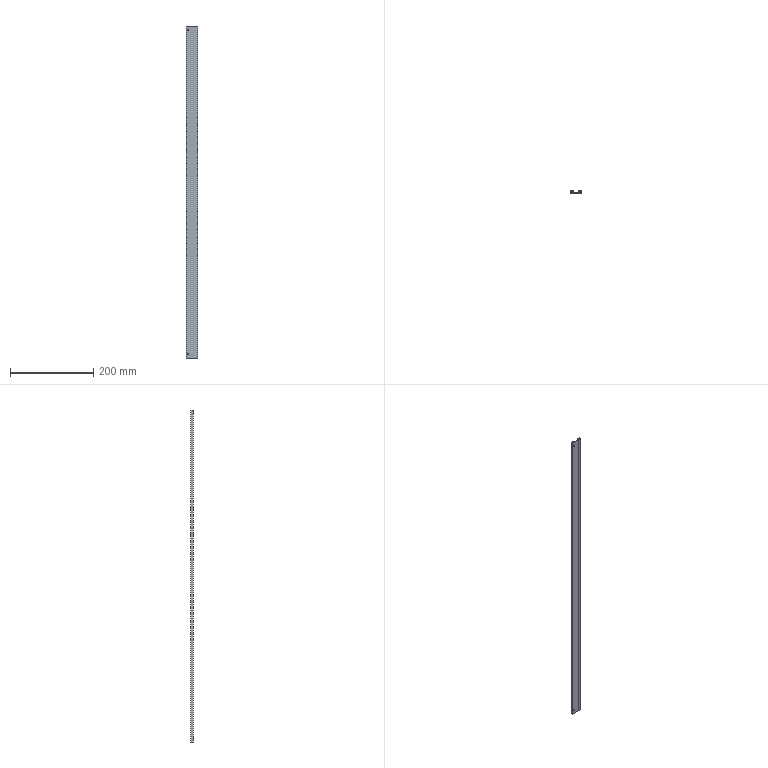Part | SolidWorks | features BossThin 1, ExtruThin 1, HoleWzd 1, MirrorSolid 1 | 1 solid | 30 faces | box 28 x 5 x 800 mm | volume 39502 mm3 | plane 26 | cylinder 4 | commonest cylinder face diameters 3.4 x4
STEP:
#1=CARTESIAN_POINT('',(-16.,0.,11.7));
#2=VERTEX_POINT('',#1);
#3=CARTESIAN_POINT('',(-16.,0.,8.3));
#4=VERTEX_POINT('',#3);
#5=CARTESIAN_POINT('',(-16.,0.,10.));
#6=DIRECTION('',(0.,-1.,0.));
#7=DIRECTION('',(0.,0.,-1.));
#8=AXIS2_PLACEMENT_3D('',#5,#6,#7);
#9=CIRCLE('',#8,1.7);
#10=EDGE_CURVE('',#2,#4,#9,.T.);
#11=ORIENTED_EDGE('',*,*,#10,.T.);
#12=CARTESIAN_POINT('',(-16.,1.,8.3));
#13=VERTEX_POINT('',#12);
#14=CARTESIAN_POINT('',(-16.,1.,8.3));
#15=DIRECTION('',(0.,1.,0.));
#16=VECTOR('',#15,1000.);
#17=LINE('',#14,#16);
#18=EDGE_CURVE('',#4,#13,#17,.T.);
#19=ORIENTED_EDGE('',*,*,#18,.T.);
#20=CARTESIAN_POINT('',(-16.,1.,11.7));
#21=VERTEX_POINT('',#20);
#22=CARTESIAN_POINT('',(-16.,1.,10.));
#23=DIRECTION('',(0.,1.,0.));
#24=DIRECTION('',(0.,0.,1.));
#25=AXIS2_PLACEMENT_3D('',#22,#23,#24);
#26=CIRCLE('',#25,1.7);
#27=EDGE_CURVE('',#13,#21,#26,.T.);
#28=ORIENTED_EDGE('',*,*,#27,.T.);
#29=CARTESIAN_POINT('',(-16.,1.,11.7));
#30=DIRECTION('',(0.,1.,0.));
#31=VECTOR('',#30,1000.);
#32=LINE('',#29,#31);
#33=EDGE_CURVE('',#2,#21,#32,.T.);
#34=ORIENTED_EDGE('',*,*,#33,.F.);
#35=EDGE_LOOP('',(#11,#19,#28,#34));
#36=FACE_OUTER_BOUND('',#35,.T.);
#37=CARTESIAN_POINT('',(-16.,1.,10.));
#38=DIRECTION('',(0.,1.,0.));
#39=DIRECTION('',(0.,0.,1.));
#40=AXIS2_PLACEMENT_3D('',#37,#38,#39);
#41=CYLINDRICAL_SURFACE('',#40,1.7);
#42=ADVANCED_FACE('',(#36),#41,.F.);
#43=CARTESIAN_POINT('',(-16.,0.,791.7));
#44=VERTEX_POINT('',#43);
#45=CARTESIAN_POINT('',(-16.,0.,788.3));
#46=VERTEX_POINT('',#45);
#47=CARTESIAN_POINT('',(-16.,0.,790.));
#48=DIRECTION('',(0.,-1.,0.));
#49=DIRECTION('',(0.,0.,-1.));
#50=AXIS2_PLACEMENT_3D('',#47,#48,#49);
#51=CIRCLE('',#50,1.7);
#52=EDGE_CURVE('',#44,#46,#51,.T.);
#53=ORIENTED_EDGE('',*,*,#52,.T.);
#54=CARTESIAN_POINT('',(-16.,1.,788.3));
#55=VERTEX_POINT('',#54);
#56=CARTESIAN_POINT('',(-16.,1.,788.3));
#57=DIRECTION('',(0.,1.,0.));
#58=VECTOR('',#57,1000.);
#59=LINE('',#56,#58);
#60=EDGE_CURVE('',#46,#55,#59,.T.);
#61=ORIENTED_EDGE('',*,*,#60,.T.);
#62=CARTESIAN_POINT('',(-16.,1.,791.7));
#63=VERTEX_POINT('',#62);
#64=CARTESIAN_POINT('',(-16.,1.,790.));
#65=DIRECTION('',(0.,1.,0.));
#66=DIRECTION('',(0.,0.,1.));
#67=AXIS2_PLACEMENT_3D('',#64,#65,#66);
#68=CIRCLE('',#67,1.7);
#69=EDGE_CURVE('',#55,#63,#68,.T.);
#70=ORIENTED_EDGE('',*,*,#69,.T.);
#71=CARTESIAN_POINT('',(-16.,1.,791.7));
#72=DIRECTION('',(0.,1.,0.));
#73=VECTOR('',#72,1000.);
#74=LINE('',#71,#73);
#75=EDGE_CURVE('',#44,#63,#74,.T.);
#76=ORIENTED_EDGE('',*,*,#75,.F.);
#77=EDGE_LOOP('',(#53,#61,#70,#76));
#78=FACE_OUTER_BOUND('',#77,.T.);
#79=CARTESIAN_POINT('',(-16.,1.,790.));
#80=DIRECTION('',(0.,1.,0.));
#81=DIRECTION('',(0.,0.,1.));
#82=AXIS2_PLACEMENT_3D('',#79,#80,#81);
#83=CYLINDRICAL_SURFACE('',#82,1.7);
#84=ADVANCED_FACE('',(#78),#83,.F.);
#85=CARTESIAN_POINT('',(0.,1.,0.));
#86=VERTEX_POINT('',#85);
#87=CARTESIAN_POINT('',(0.,5.,0.));
#88=VERTEX_POINT('',#87);
#89=CARTESIAN_POINT('',(0.,0.,0.));
#90=DIRECTION('',(0.,1.,0.));
#91=VECTOR('',#90,1000.);
#92=LINE('',#89,#91);
#93=EDGE_CURVE('',#86,#88,#92,.T.);
#94=ORIENTED_EDGE('',*,*,#93,.F.);
#95=CARTESIAN_POINT('',(0.,1.,800.));
#96=VERTEX_POINT('',#95);
#97=CARTESIAN_POINT('',(0.,1.,-6.083));
#98=DIRECTION('',(0.,0.,1.));
#99=VECTOR('',#98,1000.);
#100=LINE('',#97,#99);
#101=EDGE_CURVE('',#86,#96,#100,.T.);
#102=ORIENTED_EDGE('',*,*,#101,.T.);
#103=CARTESIAN_POINT('',(0.,5.,800.));
#104=VERTEX_POINT('',#103);
#105=CARTESIAN_POINT('',(0.,0.,800.));
#106=DIRECTION('',(0.,1.,0.));
#107=VECTOR('',#106,1000.);
#108=LINE('',#105,#107);
#109=EDGE_CURVE('',#96,#104,#108,.T.);
#110=ORIENTED_EDGE('',*,*,#109,.T.);
#111=CARTESIAN_POINT('',(0.,5.,800.));
#112=DIRECTION('',(0.,0.,-1.));
#113=VECTOR('',#112,1000.);
#114=LINE('',#111,#113);
#115=EDGE_CURVE('',#104,#88,#114,.T.);
#116=ORIENTED_EDGE('',*,*,#115,.T.);
#117=EDGE_LOOP('',(#94,#102,#110,#116));
#118=FACE_OUTER_BOUND('',#117,.T.);
#119=CARTESIAN_POINT('',(0.,0.,800.));
#120=DIRECTION('',(-1.,0.,0.));
#121=DIRECTION('',(0.,0.,1.));
#122=AXIS2_PLACEMENT_3D('',#119,#120,#121);
#123=PLANE('',#122);
#124=ADVANCED_FACE('',(#118),#123,.T.);
#125=CARTESIAN_POINT('',(1.,4.,0.));
#126=VERTEX_POINT('',#125);
#127=CARTESIAN_POINT('',(2.35,4.,0.));
#128=VERTEX_POINT('',#127);
#129=CARTESIAN_POINT('',(0.,4.,0.));
#130=DIRECTION('',(1.,0.,0.));
#131=VECTOR('',#130,1000.);
#132=LINE('',#129,#131);
#133=EDGE_CURVE('',#126,#128,#132,.T.);
#134=ORIENTED_EDGE('',*,*,#133,.T.);
#135=CARTESIAN_POINT('',(2.35,4.,800.));
#136=VERTEX_POINT('',#135);
#137=CARTESIAN_POINT('',(2.35,4.,800.));
#138=DIRECTION('',(0.,0.,-1.));
#139=VECTOR('',#138,1000.);
#140=LINE('',#137,#139);
#141=EDGE_CURVE('',#136,#128,#140,.T.);
#142=ORIENTED_EDGE('',*,*,#141,.F.);
#143=CARTESIAN_POINT('',(1.,4.,800.));
#144=VERTEX_POINT('',#143);
#145=CARTESIAN_POINT('',(0.,4.,800.));
#146=DIRECTION('',(1.,0.,0.));
#147=VECTOR('',#146,1000.);
#148=LINE('',#145,#147);
#149=EDGE_CURVE('',#144,#136,#148,.T.);
#150=ORIENTED_EDGE('',*,*,#149,.F.);
#151=CARTESIAN_POINT('',(1.,4.,800.));
#152=DIRECTION('',(0.,0.,-1.));
#153=VECTOR('',#152,1000.);
#154=LINE('',#151,#153);
#155=EDGE_CURVE('',#144,#126,#154,.T.);
#156=ORIENTED_EDGE('',*,*,#155,.T.);
#157=EDGE_LOOP('',(#134,#142,#150,#156));
#158=FACE_OUTER_BOUND('',#157,.T.);
#159=CARTESIAN_POINT('',(0.,4.,800.));
#160=DIRECTION('',(0.,1.,0.));
#161=DIRECTION('',(-1.,0.,0.));
#162=AXIS2_PLACEMENT_3D('',#159,#160,#161);
#163=PLANE('',#162);
#164=ADVANCED_FACE('',(#158),#163,.F.);
#165=CARTESIAN_POINT('',(2.35,5.,0.));
#166=VERTEX_POINT('',#165);
#167=CARTESIAN_POINT('',(2.35,5.,0.));
#168=DIRECTION('',(0.,-1.,0.));
#169=VECTOR('',#168,1000.);
#170=LINE('',#167,#169);
#171=EDGE_CURVE('',#166,#128,#170,.T.);
#172=ORIENTED_EDGE('',*,*,#171,.F.);
#173=CARTESIAN_POINT('',(2.35,5.,800.));
#174=VERTEX_POINT('',#173);
#175=CARTESIAN_POINT('',(2.35,5.,800.));
#176=DIRECTION('',(0.,0.,-1.));
#177=VECTOR('',#176,1000.);
#178=LINE('',#175,#177);
#179=EDGE_CURVE('',#174,#166,#178,.T.);
#180=ORIENTED_EDGE('',*,*,#179,.F.);
#181=CARTESIAN_POINT('',(2.35,5.,800.));
#182=DIRECTION('',(0.,-1.,0.));
#183=VECTOR('',#182,1000.);
#184=LINE('',#181,#183);
#185=EDGE_CURVE('',#174,#136,#184,.T.);
#186=ORIENTED_EDGE('',*,*,#185,.T.);
#187=ORIENTED_EDGE('',*,*,#141,.T.);
#188=EDGE_LOOP('',(#172,#180,#186,#187));
#189=FACE_OUTER_BOUND('',#188,.T.);
#190=CARTESIAN_POINT('',(2.35,5.,800.));
#191=DIRECTION('',(1.,0.,0.));
#192=DIRECTION('',(0.,1.,0.));
#193=AXIS2_PLACEMENT_3D('',#190,#191,#192);
#194=PLANE('',#193);
#195=ADVANCED_FACE('',(#189),#194,.T.);
#196=CARTESIAN_POINT('',(0.,5.,0.));
#197=DIRECTION('',(1.,0.,0.));
#198=VECTOR('',#197,1000.);
#199=LINE('',#196,#198);
#200=EDGE_CURVE('',#88,#166,#199,.T.);
#201=ORIENTED_EDGE('',*,*,#200,.F.);
#202=ORIENTED_EDGE('',*,*,#115,.F.);
#203=CARTESIAN_POINT('',(0.,5.,800.));
#204=DIRECTION('',(1.,0.,0.));
#205=VECTOR('',#204,1000.);
#206=LINE('',#203,#205);
#207=EDGE_CURVE('',#104,#174,#206,.T.);
#208=ORIENTED_EDGE('',*,*,#207,.T.);
#209=ORIENTED_EDGE('',*,*,#179,.T.);
#210=EDGE_LOOP('',(#201,#202,#208,#209));
#211=FACE_OUTER_BOUND('',#210,.T.);
#212=CARTESIAN_POINT('',(0.,5.,800.));
#213=DIRECTION('',(0.,1.,0.));
#214=DIRECTION('',(-1.,0.,0.));
#215=AXIS2_PLACEMENT_3D('',#212,#213,#214);
#216=PLANE('',#215);
#217=ADVANCED_FACE('',(#211),#216,.T.);
#218=ORIENTED_EDGE('',*,*,#10,.F.);
#219=CARTESIAN_POINT('',(-16.,0.,10.));
#220=DIRECTION('',(0.,-1.,0.));
#221=DIRECTION('',(0.,0.,-1.));
#222=AXIS2_PLACEMENT_3D('',#219,#220,#221);
#223=CIRCLE('',#222,1.7);
#224=EDGE_CURVE('',#4,#2,#223,.T.);
#225=ORIENTED_EDGE('',*,*,#224,.F.);
#226=EDGE_LOOP('',(#218,#225));
#227=FACE_BOUND('',#226,.T.);
#228=ORIENTED_EDGE('',*,*,#52,.F.);
#229=CARTESIAN_POINT('',(-16.,0.,790.));
#230=DIRECTION('',(0.,-1.,0.));
#231=DIRECTION('',(0.,0.,-1.));
#232=AXIS2_PLACEMENT_3D('',#229,#230,#231);
#233=CIRCLE('',#232,1.7);
#234=EDGE_CURVE('',#46,#44,#233,.T.);
#235=ORIENTED_EDGE('',*,*,#234,.F.);
#236=EDGE_LOOP('',(#228,#235));
#237=FACE_BOUND('',#236,.T.);
#238=CARTESIAN_POINT('',(8.,0.,0.));
#239=VERTEX_POINT('',#238);
#240=CARTESIAN_POINT('',(-20.,0.,0.));
#241=VERTEX_POINT('',#240);
#242=CARTESIAN_POINT('',(0.,0.,0.));
#243=DIRECTION('',(-1.,0.,0.));
#244=VECTOR('',#243,1000.);
#245=LINE('',#242,#244);
#246=EDGE_CURVE('',#239,#241,#245,.T.);
#247=ORIENTED_EDGE('',*,*,#246,.F.);
#248=CARTESIAN_POINT('',(8.,0.,800.));
#249=VERTEX_POINT('',#248);
#250=CARTESIAN_POINT('',(8.,0.,800.));
#251=DIRECTION('',(0.,0.,-1.));
#252=VECTOR('',#251,1000.);
#253=LINE('',#250,#252);
#254=EDGE_CURVE('',#249,#239,#253,.T.);
#255=ORIENTED_EDGE('',*,*,#254,.F.);
#256=CARTESIAN_POINT('',(-20.,0.,800.));
#257=VERTEX_POINT('',#256);
#258=CARTESIAN_POINT('',(0.,0.,800.));
#259=DIRECTION('',(-1.,0.,0.));
#260=VECTOR('',#259,1000.);
#261=LINE('',#258,#260);
#262=EDGE_CURVE('',#249,#257,#261,.T.);
#263=ORIENTED_EDGE('',*,*,#262,.T.);
#264=CARTESIAN_POINT('',(-20.,0.,800.));
#265=DIRECTION('',(0.,0.,-1.));
#266=VECTOR('',#265,1000.);
#267=LINE('',#264,#266);
#268=EDGE_CURVE('',#257,#241,#267,.T.);
#269=ORIENTED_EDGE('',*,*,#268,.T.);
#270=EDGE_LOOP('',(#247,#255,#263,#269));
#271=FACE_OUTER_BOUND('',#270,.T.);
#272=CARTESIAN_POINT('',(0.,0.,800.));
#273=DIRECTION('',(0.,-1.,0.));
#274=DIRECTION('',(0.,0.,-1.));
#275=AXIS2_PLACEMENT_3D('',#272,#273,#274);
#276=PLANE('',#275);
#277=ADVANCED_FACE('',(#227,#237,#271),#276,.T.);
#278=CARTESIAN_POINT('',(8.,5.,0.));
#279=VERTEX_POINT('',#278);
#280=CARTESIAN_POINT('',(8.,0.,0.));
#281=DIRECTION('',(0.,-1.,0.));
#282=VECTOR('',#281,1000.);
#283=LINE('',#280,#282);
#284=EDGE_CURVE('',#279,#239,#283,.T.);
#285=ORIENTED_EDGE('',*,*,#284,.F.);
#286=CARTESIAN_POINT('',(8.,5.,800.));
#287=VERTEX_POINT('',#286);
#288=CARTESIAN_POINT('',(8.,5.,800.));
#289=DIRECTION('',(0.,0.,-1.));
#290=VECTOR('',#289,1000.);
#291=LINE('',#288,#290);
#292=EDGE_CURVE('',#287,#279,#291,.T.);
#293=ORIENTED_EDGE('',*,*,#292,.F.);
#294=CARTESIAN_POINT('',(8.,0.,800.));
#295=DIRECTION('',(0.,-1.,0.));
#296=VECTOR('',#295,1000.);
#297=LINE('',#294,#296);
#298=EDGE_CURVE('',#287,#249,#297,.T.);
#299=ORIENTED_EDGE('',*,*,#298,.T.);
#300=ORIENTED_EDGE('',*,*,#254,.T.);
#301=EDGE_LOOP('',(#285,#293,#299,#300));
#302=FACE_OUTER_BOUND('',#301,.T.);
#303=CARTESIAN_POINT('',(8.,0.,800.));
#304=DIRECTION('',(1.,0.,0.));
#305=DIRECTION('',(0.,0.,-1.));
#306=AXIS2_PLACEMENT_3D('',#303,#304,#305);
#307=PLANE('',#306);
#308=ADVANCED_FACE('',(#302),#307,.T.);
#309=CARTESIAN_POINT('',(5.65,5.,0.));
#310=VERTEX_POINT('',#309);
#311=CARTESIAN_POINT('',(8.,5.,0.));
#312=DIRECTION('',(1.,0.,0.));
#313=VECTOR('',#312,1000.);
#314=LINE('',#311,#313);
#315=EDGE_CURVE('',#310,#279,#314,.T.);
#316=ORIENTED_EDGE('',*,*,#315,.F.);
#317=CARTESIAN_POINT('',(5.65,5.,800.));
#318=VERTEX_POINT('',#317);
#319=CARTESIAN_POINT('',(5.65,5.,800.));
#320=DIRECTION('',(0.,0.,-1.));
#321=VECTOR('',#320,1000.);
#322=LINE('',#319,#321);
#323=EDGE_CURVE('',#318,#310,#322,.T.);
#324=ORIENTED_EDGE('',*,*,#323,.F.);
#325=CARTESIAN_POINT('',(8.,5.,800.));
#326=DIRECTION('',(1.,0.,0.));
#327=VECTOR('',#326,1000.);
#328=LINE('',#325,#327);
#329=EDGE_CURVE('',#318,#287,#328,.T.);
#330=ORIENTED_EDGE('',*,*,#329,.T.);
#331=ORIENTED_EDGE('',*,*,#292,.T.);
#332=EDGE_LOOP('',(#316,#324,#330,#331));
#333=FACE_OUTER_BOUND('',#332,.T.);
#334=CARTESIAN_POINT('',(8.,5.,800.));
#335=DIRECTION('',(0.,1.,0.));
#336=DIRECTION('',(-1.,0.,0.));
#337=AXIS2_PLACEMENT_3D('',#334,#335,#336);
#338=PLANE('',#337);
#339=ADVANCED_FACE('',(#333),#338,.T.);
#340=CARTESIAN_POINT('',(5.65,4.,0.));
#341=VERTEX_POINT('',#340);
#342=CARTESIAN_POINT('',(5.65,4.,0.));
#343=DIRECTION('',(0.,1.,0.));
#344=VECTOR('',#343,1000.);
#345=LINE('',#342,#344);
#346=EDGE_CURVE('',#341,#310,#345,.T.);
#347=ORIENTED_EDGE('',*,*,#346,.F.);
#348=CARTESIAN_POINT('',(5.65,4.,800.));
#349=VERTEX_POINT('',#348);
#350=CARTESIAN_POINT('',(5.65,4.,800.));
#351=DIRECTION('',(0.,0.,-1.));
#352=VECTOR('',#351,1000.);
#353=LINE('',#350,#352);
#354=EDGE_CURVE('',#349,#341,#353,.T.);
#355=ORIENTED_EDGE('',*,*,#354,.F.);
#356=CARTESIAN_POINT('',(5.65,4.,800.));
#357=DIRECTION('',(0.,1.,0.));
#358=VECTOR('',#357,1000.);
#359=LINE('',#356,#358);
#360=EDGE_CURVE('',#349,#318,#359,.T.);
#361=ORIENTED_EDGE('',*,*,#360,.T.);
#362=ORIENTED_EDGE('',*,*,#323,.T.);
#363=EDGE_LOOP('',(#347,#355,#361,#362));
#364=FACE_OUTER_BOUND('',#363,.T.);
#365=CARTESIAN_POINT('',(5.65,4.,800.));
#366=DIRECTION('',(-1.,0.,0.));
#367=DIRECTION('',(0.,0.,1.));
#368=AXIS2_PLACEMENT_3D('',#365,#366,#367);
#369=PLANE('',#368);
#370=ADVANCED_FACE('',(#364),#369,.T.);
#371=CARTESIAN_POINT('',(7.,4.,0.));
#372=VERTEX_POINT('',#371);
#373=CARTESIAN_POINT('',(8.,4.,0.));
#374=DIRECTION('',(1.,0.,0.));
#375=VECTOR('',#374,1000.);
#376=LINE('',#373,#375);
#377=EDGE_CURVE('',#341,#372,#376,.T.);
#378=ORIENTED_EDGE('',*,*,#377,.T.);
#379=CARTESIAN_POINT('',(7.,4.,800.));
#380=VERTEX_POINT('',#379);
#381=CARTESIAN_POINT('',(7.,4.,800.));
#382=DIRECTION('',(0.,0.,-1.));
#383=VECTOR('',#382,1000.);
#384=LINE('',#381,#383);
#385=EDGE_CURVE('',#380,#372,#384,.T.);
#386=ORIENTED_EDGE('',*,*,#385,.F.);
#387=CARTESIAN_POINT('',(8.,4.,800.));
#388=DIRECTION('',(1.,0.,0.));
#389=VECTOR('',#388,1000.);
#390=LINE('',#387,#389);
#391=EDGE_CURVE('',#349,#380,#390,.T.);
#392=ORIENTED_EDGE('',*,*,#391,.F.);
#393=ORIENTED_EDGE('',*,*,#354,.T.);
#394=EDGE_LOOP('',(#378,#386,#392,#393));
#395=FACE_OUTER_BOUND('',#394,.T.);
#396=CARTESIAN_POINT('',(8.,4.,800.));
#397=DIRECTION('',(0.,1.,0.));
#398=DIRECTION('',(-1.,0.,0.));
#399=AXIS2_PLACEMENT_3D('',#396,#397,#398);
#400=PLANE('',#399);
#401=ADVANCED_FACE('',(#395),#400,.F.);
#402=CARTESIAN_POINT('',(7.,1.,0.));
#403=VERTEX_POINT('',#402);
#404=CARTESIAN_POINT('',(7.,0.,0.));
#405=DIRECTION('',(0.,-1.,0.));
#406=VECTOR('',#405,1000.);
#407=LINE('',#404,#406);
#408=EDGE_CURVE('',#372,#403,#407,.T.);
#409=ORIENTED_EDGE('',*,*,#408,.T.);
#410=CARTESIAN_POINT('',(7.,1.,800.));
#411=VERTEX_POINT('',#410);
#412=CARTESIAN_POINT('',(7.,1.,800.));
#413=DIRECTION('',(0.,0.,-1.));
#414=VECTOR('',#413,1000.);
#415=LINE('',#412,#414);
#416=EDGE_CURVE('',#411,#403,#415,.T.);
#417=ORIENTED_EDGE('',*,*,#416,.F.);
#418=CARTESIAN_POINT('',(7.,0.,800.));
#419=DIRECTION('',(0.,-1.,0.));
#420=VECTOR('',#419,1000.);
#421=LINE('',#418,#420);
#422=EDGE_CURVE('',#380,#411,#421,.T.);
#423=ORIENTED_EDGE('',*,*,#422,.F.);
#424=ORIENTED_EDGE('',*,*,#385,.T.);
#425=EDGE_LOOP('',(#409,#417,#423,#424));
#426=FACE_OUTER_BOUND('',#425,.T.);
#427=CARTESIAN_POINT('',(7.,0.,800.));
#428=DIRECTION('',(1.,0.,0.));
#429=DIRECTION('',(0.,0.,-1.));
#430=AXIS2_PLACEMENT_3D('',#427,#428,#429);
#431=PLANE('',#430);
#432=ADVANCED_FACE('',(#426),#431,.F.);
#433=CARTESIAN_POINT('',(1.,1.,0.));
#434=VERTEX_POINT('',#433);
#435=CARTESIAN_POINT('',(0.,1.,0.));
#436=DIRECTION('',(-1.,0.,0.));
#437=VECTOR('',#436,1000.);
#438=LINE('',#435,#437);
#439=EDGE_CURVE('',#403,#434,#438,.T.);
#440=ORIENTED_EDGE('',*,*,#439,.T.);
#441=CARTESIAN_POINT('',(1.,1.,800.));
#442=VERTEX_POINT('',#441);
#443=CARTESIAN_POINT('',(1.,1.,800.));
#444=DIRECTION('',(0.,0.,-1.));
#445=VECTOR('',#444,1000.);
#446=LINE('',#443,#445);
#447=EDGE_CURVE('',#442,#434,#446,.T.);
#448=ORIENTED_EDGE('',*,*,#447,.F.);
#449=CARTESIAN_POINT('',(0.,1.,800.));
#450=DIRECTION('',(-1.,0.,0.));
#451=VECTOR('',#450,1000.);
#452=LINE('',#449,#451);
#453=EDGE_CURVE('',#411,#442,#452,.T.);
#454=ORIENTED_EDGE('',*,*,#453,.F.);
#455=ORIENTED_EDGE('',*,*,#416,.T.);
#456=EDGE_LOOP('',(#440,#448,#454,#455));
#457=FACE_OUTER_BOUND('',#456,.T.);
#458=CARTESIAN_POINT('',(0.,1.,800.));
#459=DIRECTION('',(0.,-1.,0.));
#460=DIRECTION('',(0.,0.,-1.));
#461=AXIS2_PLACEMENT_3D('',#458,#459,#460);
#462=PLANE('',#461);
#463=ADVANCED_FACE('',(#457),#462,.F.);
#464=CARTESIAN_POINT('',(1.,0.,0.));
#465=DIRECTION('',(0.,1.,0.));
#466=VECTOR('',#465,1000.);
#467=LINE('',#464,#466);
#468=EDGE_CURVE('',#434,#126,#467,.T.);
#469=ORIENTED_EDGE('',*,*,#468,.T.);
#470=ORIENTED_EDGE('',*,*,#155,.F.);
#471=CARTESIAN_POINT('',(1.,0.,800.));
#472=DIRECTION('',(0.,1.,0.));
#473=VECTOR('',#472,1000.);
#474=LINE('',#471,#473);
#475=EDGE_CURVE('',#442,#144,#474,.T.);
#476=ORIENTED_EDGE('',*,*,#475,.F.);
#477=ORIENTED_EDGE('',*,*,#447,.T.);
#478=EDGE_LOOP('',(#469,#470,#476,#477));
#479=FACE_OUTER_BOUND('',#478,.T.);
#480=CARTESIAN_POINT('',(1.,0.,800.));
#481=DIRECTION('',(-1.,0.,0.));
#482=DIRECTION('',(0.,0.,1.));
#483=AXIS2_PLACEMENT_3D('',#480,#481,#482);
#484=PLANE('',#483);
#485=ADVANCED_FACE('',(#479),#484,.F.);
#486=ORIENTED_EDGE('',*,*,#149,.T.);
#487=ORIENTED_EDGE('',*,*,#185,.F.);
#488=ORIENTED_EDGE('',*,*,#207,.F.);
#489=ORIENTED_EDGE('',*,*,#109,.F.);
#490=CARTESIAN_POINT('',(-12.,1.,800.));
#491=VERTEX_POINT('',#490);
#492=CARTESIAN_POINT('',(0.,1.,800.));
#493=DIRECTION('',(-1.,0.,0.));
#494=VECTOR('',#493,1000.);
#495=LINE('',#492,#494);
#496=EDGE_CURVE('',#96,#491,#495,.T.);
#497=ORIENTED_EDGE('',*,*,#496,.T.);
#498=CARTESIAN_POINT('',(-12.,5.,800.));
#499=VERTEX_POINT('',#498);
#500=CARTESIAN_POINT('',(-12.,0.,800.));
#501=DIRECTION('',(0.,1.,0.));
#502=VECTOR('',#501,1000.);
#503=LINE('',#500,#502);
#504=EDGE_CURVE('',#491,#499,#503,.T.);
#505=ORIENTED_EDGE('',*,*,#504,.T.);
#506=CARTESIAN_POINT('',(-14.35,5.,800.));
#507=VERTEX_POINT('',#506);
#508=CARTESIAN_POINT('',(-12.,5.,800.));
#509=DIRECTION('',(-1.,0.,0.));
#510=VECTOR('',#509,1000.);
#511=LINE('',#508,#510);
#512=EDGE_CURVE('',#499,#507,#511,.T.);
#513=ORIENTED_EDGE('',*,*,#512,.T.);
#514=CARTESIAN_POINT('',(-14.35,4.,800.));
#515=VERTEX_POINT('',#514);
#516=CARTESIAN_POINT('',(-14.35,5.,800.));
#517=DIRECTION('',(0.,-1.,0.));
#518=VECTOR('',#517,1000.);
#519=LINE('',#516,#518);
#520=EDGE_CURVE('',#507,#515,#519,.T.);
#521=ORIENTED_EDGE('',*,*,#520,.T.);
#522=CARTESIAN_POINT('',(-13.,4.,800.));
#523=VERTEX_POINT('',#522);
#524=CARTESIAN_POINT('',(-12.,4.,800.));
#525=DIRECTION('',(-1.,0.,0.));
#526=VECTOR('',#525,1000.);
#527=LINE('',#524,#526);
#528=EDGE_CURVE('',#523,#515,#527,.T.);
#529=ORIENTED_EDGE('',*,*,#528,.F.);
#530=CARTESIAN_POINT('',(-13.,1.,800.));
#531=VERTEX_POINT('',#530);
#532=CARTESIAN_POINT('',(-13.,0.,800.));
#533=DIRECTION('',(0.,1.,0.));
#534=VECTOR('',#533,1000.);
#535=LINE('',#532,#534);
#536=EDGE_CURVE('',#531,#523,#535,.T.);
#537=ORIENTED_EDGE('',*,*,#536,.F.);
#538=CARTESIAN_POINT('',(-19.,1.,800.));
#539=VERTEX_POINT('',#538);
#540=CARTESIAN_POINT('',(-12.,1.,800.));
#541=DIRECTION('',(1.,0.,0.));
#542=VECTOR('',#541,1000.);
#543=LINE('',#540,#542);
#544=EDGE_CURVE('',#539,#531,#543,.T.);
#545=ORIENTED_EDGE('',*,*,#544,.F.);
#546=CARTESIAN_POINT('',(-19.,4.,800.));
#547=VERTEX_POINT('',#546);
#548=CARTESIAN_POINT('',(-19.,0.,800.));
#549=DIRECTION('',(0.,-1.,0.));
#550=VECTOR('',#549,1000.);
#551=LINE('',#548,#550);
#552=EDGE_CURVE('',#547,#539,#551,.T.);
#553=ORIENTED_EDGE('',*,*,#552,.F.);
#554=CARTESIAN_POINT('',(-17.65,4.,800.));
#555=VERTEX_POINT('',#554);
#556=CARTESIAN_POINT('',(-20.,4.,800.));
#557=DIRECTION('',(-1.,0.,0.));
#558=VECTOR('',#557,1000.);
#559=LINE('',#556,#558);
#560=EDGE_CURVE('',#555,#547,#559,.T.);
#561=ORIENTED_EDGE('',*,*,#560,.F.);
#562=CARTESIAN_POINT('',(-17.65,5.,800.));
#563=VERTEX_POINT('',#562);
#564=CARTESIAN_POINT('',(-17.65,4.,800.));
#565=DIRECTION('',(0.,1.,0.));
#566=VECTOR('',#565,1000.);
#567=LINE('',#564,#566);
#568=EDGE_CURVE('',#555,#563,#567,.T.);
#569=ORIENTED_EDGE('',*,*,#568,.T.);
#570=CARTESIAN_POINT('',(-20.,5.,800.));
#571=VERTEX_POINT('',#570);
#572=CARTESIAN_POINT('',(-20.,5.,800.));
#573=DIRECTION('',(-1.,0.,0.));
#574=VECTOR('',#573,1000.);
#575=LINE('',#572,#574);
#576=EDGE_CURVE('',#563,#571,#575,.T.);
#577=ORIENTED_EDGE('',*,*,#576,.T.);
#578=CARTESIAN_POINT('',(-20.,0.,800.));
#579=DIRECTION('',(0.,-1.,0.));
#580=VECTOR('',#579,1000.);
#581=LINE('',#578,#580);
#582=EDGE_CURVE('',#571,#257,#581,.T.);
#583=ORIENTED_EDGE('',*,*,#582,.T.);
#584=ORIENTED_EDGE('',*,*,#262,.F.);
#585=ORIENTED_EDGE('',*,*,#298,.F.);
#586=ORIENTED_EDGE('',*,*,#329,.F.);
#587=ORIENTED_EDGE('',*,*,#360,.F.);
#588=ORIENTED_EDGE('',*,*,#391,.T.);
#589=ORIENTED_EDGE('',*,*,#422,.T.);
#590=ORIENTED_EDGE('',*,*,#453,.T.);
#591=ORIENTED_EDGE('',*,*,#475,.T.);
#592=EDGE_LOOP('',(#486,#487,#488,#489,#497,#505,#513,#521,#529,#537,#545,#553,#561,#569,#577,#583,#584,#585,#586,#587,#588,#589,#590,#591));
#593=FACE_OUTER_BOUND('',#592,.T.);
#594=CARTESIAN_POINT('',(0.,0.,800.));
#595=DIRECTION('',(0.,0.,-1.));
#596=DIRECTION('',(-1.,0.,0.));
#597=AXIS2_PLACEMENT_3D('',#594,#595,#596);
#598=PLANE('',#597);
#599=ADVANCED_FACE('',(#593),#598,.F.);
#600=ORIENTED_EDGE('',*,*,#133,.F.);
#601=ORIENTED_EDGE('',*,*,#468,.F.);
#602=ORIENTED_EDGE('',*,*,#439,.F.);
#603=ORIENTED_EDGE('',*,*,#408,.F.);
#604=ORIENTED_EDGE('',*,*,#377,.F.);
#605=ORIENTED_EDGE('',*,*,#346,.T.);
#606=ORIENTED_EDGE('',*,*,#315,.T.);
#607=ORIENTED_EDGE('',*,*,#284,.T.);
#608=ORIENTED_EDGE('',*,*,#246,.T.);
#609=CARTESIAN_POINT('',(-20.,5.,0.));
#610=VERTEX_POINT('',#609);
#611=CARTESIAN_POINT('',(-20.,0.,0.));
#612=DIRECTION('',(0.,-1.,0.));
#613=VECTOR('',#612,1000.);
#614=LINE('',#611,#613);
#615=EDGE_CURVE('',#610,#241,#614,.T.);
#616=ORIENTED_EDGE('',*,*,#615,.F.);
#617=CARTESIAN_POINT('',(-17.65,5.,0.));
#618=VERTEX_POINT('',#617);
#619=CARTESIAN_POINT('',(-20.,5.,0.));
#620=DIRECTION('',(-1.,0.,0.));
#621=VECTOR('',#620,1000.);
#622=LINE('',#619,#621);
#623=EDGE_CURVE('',#618,#610,#622,.T.);
#624=ORIENTED_EDGE('',*,*,#623,.F.);
#625=CARTESIAN_POINT('',(-17.65,4.,0.));
#626=VERTEX_POINT('',#625);
#627=CARTESIAN_POINT('',(-17.65,4.,0.));
#628=DIRECTION('',(0.,1.,0.));
#629=VECTOR('',#628,1000.);
#630=LINE('',#627,#629);
#631=EDGE_CURVE('',#626,#618,#630,.T.);
#632=ORIENTED_EDGE('',*,*,#631,.F.);
#633=CARTESIAN_POINT('',(-19.,4.,0.));
#634=VERTEX_POINT('',#633);
#635=CARTESIAN_POINT('',(-20.,4.,0.));
#636=DIRECTION('',(-1.,0.,0.));
#637=VECTOR('',#636,1000.);
#638=LINE('',#635,#637);
#639=EDGE_CURVE('',#626,#634,#638,.T.);
#640=ORIENTED_EDGE('',*,*,#639,.T.);
#641=CARTESIAN_POINT('',(-19.,1.,0.));
#642=VERTEX_POINT('',#641);
#643=CARTESIAN_POINT('',(-19.,0.,0.));
#644=DIRECTION('',(0.,-1.,0.));
#645=VECTOR('',#644,1000.);
#646=LINE('',#643,#645);
#647=EDGE_CURVE('',#634,#642,#646,.T.);
#648=ORIENTED_EDGE('',*,*,#647,.T.);
#649=CARTESIAN_POINT('',(-13.,1.,0.));
#650=VERTEX_POINT('',#649);
#651=CARTESIAN_POINT('',(-12.,1.,0.));
#652=DIRECTION('',(1.,0.,0.));
#653=VECTOR('',#652,1000.);
#654=LINE('',#651,#653);
#655=EDGE_CURVE('',#642,#650,#654,.T.);
#656=ORIENTED_EDGE('',*,*,#655,.T.);
#657=CARTESIAN_POINT('',(-13.,4.,0.));
#658=VERTEX_POINT('',#657);
#659=CARTESIAN_POINT('',(-13.,0.,0.));
#660=DIRECTION('',(0.,1.,0.));
#661=VECTOR('',#660,1000.);
#662=LINE('',#659,#661);
#663=EDGE_CURVE('',#650,#658,#662,.T.);
#664=ORIENTED_EDGE('',*,*,#663,.T.);
#665=CARTESIAN_POINT('',(-14.35,4.,0.));
#666=VERTEX_POINT('',#665);
#667=CARTESIAN_POINT('',(-12.,4.,0.));
#668=DIRECTION('',(-1.,0.,0.));
#669=VECTOR('',#668,1000.);
#670=LINE('',#667,#669);
#671=EDGE_CURVE('',#658,#666,#670,.T.);
#672=ORIENTED_EDGE('',*,*,#671,.T.);
#673=CARTESIAN_POINT('',(-14.35,5.,0.));
#674=VERTEX_POINT('',#673);
#675=CARTESIAN_POINT('',(-14.35,5.,0.));
#676=DIRECTION('',(0.,-1.,0.));
#677=VECTOR('',#676,1000.);
#678=LINE('',#675,#677);
#679=EDGE_CURVE('',#674,#666,#678,.T.);
#680=ORIENTED_EDGE('',*,*,#679,.F.);
#681=CARTESIAN_POINT('',(-12.,5.,0.));
#682=VERTEX_POINT('',#681);
#683=CARTESIAN_POINT('',(-12.,5.,0.));
#684=DIRECTION('',(-1.,0.,0.));
#685=VECTOR('',#684,1000.);
#686=LINE('',#683,#685);
#687=EDGE_CURVE('',#682,#674,#686,.T.);
#688=ORIENTED_EDGE('',*,*,#687,.F.);
#689=CARTESIAN_POINT('',(-12.,1.,0.));
#690=VERTEX_POINT('',#689);
#691=CARTESIAN_POINT('',(-12.,0.,0.));
#692=DIRECTION('',(0.,1.,0.));
#693=VECTOR('',#692,1000.);
#694=LINE('',#691,#693);
#695=EDGE_CURVE('',#690,#682,#694,.T.);
#696=ORIENTED_EDGE('',*,*,#695,.F.);
#697=CARTESIAN_POINT('',(0.,1.,0.));
#698=DIRECTION('',(-1.,0.,0.));
#699=VECTOR('',#698,1000.);
#700=LINE('',#697,#699);
#701=EDGE_CURVE('',#86,#690,#700,.T.);
#702=ORIENTED_EDGE('',*,*,#701,.F.);
#703=ORIENTED_EDGE('',*,*,#93,.T.);
#704=ORIENTED_EDGE('',*,*,#200,.T.);
#705=ORIENTED_EDGE('',*,*,#171,.T.);
#706=EDGE_LOOP('',(#600,#601,#602,#603,#604,#605,#606,#607,#608,#616,#624,#632,#640,#648,#656,#664,#672,#680,#688,#696,#702,#703,#704,#705));
#707=FACE_OUTER_BOUND('',#706,.T.);
#708=CARTESIAN_POINT('',(0.,0.,0.));
#709=DIRECTION('',(0.,0.,-1.));
#710=DIRECTION('',(-1.,0.,0.));
#711=AXIS2_PLACEMENT_3D('',#708,#709,#710);
#712=PLANE('',#711);
#713=ADVANCED_FACE('',(#707),#712,.T.);
#714=ORIENTED_EDGE('',*,*,#101,.F.);
#715=ORIENTED_EDGE('',*,*,#701,.T.);
#716=CARTESIAN_POINT('',(-12.,1.,-6.083));
#717=DIRECTION('',(0.,0.,1.));
#718=VECTOR('',#717,1000.);
#719=LINE('',#716,#718);
#720=EDGE_CURVE('',#690,#491,#719,.T.);
#721=ORIENTED_EDGE('',*,*,#720,.T.);
#722=ORIENTED_EDGE('',*,*,#496,.F.);
#723=EDGE_LOOP('',(#714,#715,#721,#722));
#724=FACE_OUTER_BOUND('',#723,.T.);
#725=CARTESIAN_POINT('',(0.,1.,-6.083));
#726=DIRECTION('',(0.,1.,0.));
#727=DIRECTION('',(-1.,0.,0.));
#728=AXIS2_PLACEMENT_3D('',#725,#726,#727);
#729=PLANE('',#728);
#730=ADVANCED_FACE('',(#724),#729,.T.);
#731=ORIENTED_EDGE('',*,*,#695,.T.);
#732=CARTESIAN_POINT('',(-12.,5.,800.));
#733=DIRECTION('',(0.,0.,-1.));
#734=VECTOR('',#733,1000.);
#735=LINE('',#732,#734);
#736=EDGE_CURVE('',#499,#682,#735,.T.);
#737=ORIENTED_EDGE('',*,*,#736,.F.);
#738=ORIENTED_EDGE('',*,*,#504,.F.);
#739=ORIENTED_EDGE('',*,*,#720,.F.);
#740=EDGE_LOOP('',(#731,#737,#738,#739));
#741=FACE_OUTER_BOUND('',#740,.T.);
#742=CARTESIAN_POINT('',(-12.,0.,800.));
#743=DIRECTION('',(1.,0.,0.));
#744=DIRECTION('',(0.,0.,1.));
#745=AXIS2_PLACEMENT_3D('',#742,#743,#744);
#746=PLANE('',#745);
#747=ADVANCED_FACE('',(#741),#746,.T.);
#748=ORIENTED_EDGE('',*,*,#671,.F.);
#749=CARTESIAN_POINT('',(-13.,4.,800.));
#750=DIRECTION('',(0.,0.,-1.));
#751=VECTOR('',#750,1000.);
#752=LINE('',#749,#751);
#753=EDGE_CURVE('',#523,#658,#752,.T.);
#754=ORIENTED_EDGE('',*,*,#753,.F.);
#755=ORIENTED_EDGE('',*,*,#528,.T.);
#756=CARTESIAN_POINT('',(-14.35,4.,800.));
#757=DIRECTION('',(0.,0.,-1.));
#758=VECTOR('',#757,1000.);
#759=LINE('',#756,#758);
#760=EDGE_CURVE('',#515,#666,#759,.T.);
#761=ORIENTED_EDGE('',*,*,#760,.T.);
#762=EDGE_LOOP('',(#748,#754,#755,#761));
#763=FACE_OUTER_BOUND('',#762,.T.);
#764=CARTESIAN_POINT('',(-12.,4.,800.));
#765=DIRECTION('',(0.,1.,0.));
#766=DIRECTION('',(1.,0.,0.));
#767=AXIS2_PLACEMENT_3D('',#764,#765,#766);
#768=PLANE('',#767);
#769=ADVANCED_FACE('',(#763),#768,.F.);
#770=ORIENTED_EDGE('',*,*,#679,.T.);
#771=ORIENTED_EDGE('',*,*,#760,.F.);
#772=ORIENTED_EDGE('',*,*,#520,.F.);
#773=CARTESIAN_POINT('',(-14.35,5.,800.));
#774=DIRECTION('',(0.,0.,-1.));
#775=VECTOR('',#774,1000.);
#776=LINE('',#773,#775);
#777=EDGE_CURVE('',#507,#674,#776,.T.);
#778=ORIENTED_EDGE('',*,*,#777,.T.);
#779=EDGE_LOOP('',(#770,#771,#772,#778));
#780=FACE_OUTER_BOUND('',#779,.T.);
#781=CARTESIAN_POINT('',(-14.35,5.,800.));
#782=DIRECTION('',(-1.,0.,0.));
#783=DIRECTION('',(0.,1.,0.));
#784=AXIS2_PLACEMENT_3D('',#781,#782,#783);
#785=PLANE('',#784);
#786=ADVANCED_FACE('',(#780),#785,.T.);
#787=ORIENTED_EDGE('',*,*,#687,.T.);
#788=ORIENTED_EDGE('',*,*,#777,.F.);
#789=ORIENTED_EDGE('',*,*,#512,.F.);
#790=ORIENTED_EDGE('',*,*,#736,.T.);
#791=EDGE_LOOP('',(#787,#788,#789,#790));
#792=FACE_OUTER_BOUND('',#791,.T.);
#793=CARTESIAN_POINT('',(-12.,5.,800.));
#794=DIRECTION('',(0.,1.,0.));
#795=DIRECTION('',(1.,0.,0.));
#796=AXIS2_PLACEMENT_3D('',#793,#794,#795);
#797=PLANE('',#796);
#798=ADVANCED_FACE('',(#792),#797,.T.);
#799=ORIENTED_EDGE('',*,*,#615,.T.);
#800=ORIENTED_EDGE('',*,*,#268,.F.);
#801=ORIENTED_EDGE('',*,*,#582,.F.);
#802=CARTESIAN_POINT('',(-20.,5.,800.));
#803=DIRECTION('',(0.,0.,-1.));
#804=VECTOR('',#803,1000.);
#805=LINE('',#802,#804);
#806=EDGE_CURVE('',#571,#610,#805,.T.);
#807=ORIENTED_EDGE('',*,*,#806,.T.);
#808=EDGE_LOOP('',(#799,#800,#801,#807));
#809=FACE_OUTER_BOUND('',#808,.T.);
#810=CARTESIAN_POINT('',(-20.,0.,800.));
#811=DIRECTION('',(-1.,0.,0.));
#812=DIRECTION('',(0.,0.,-1.));
#813=AXIS2_PLACEMENT_3D('',#810,#811,#812);
#814=PLANE('',#813);
#815=ADVANCED_FACE('',(#809),#814,.T.);
#816=ORIENTED_EDGE('',*,*,#623,.T.);
#817=ORIENTED_EDGE('',*,*,#806,.F.);
#818=ORIENTED_EDGE('',*,*,#576,.F.);
#819=CARTESIAN_POINT('',(-17.65,5.,800.));
#820=DIRECTION('',(0.,0.,-1.));
#821=VECTOR('',#820,1000.);
#822=LINE('',#819,#821);
#823=EDGE_CURVE('',#563,#618,#822,.T.);
#824=ORIENTED_EDGE('',*,*,#823,.T.);
#825=EDGE_LOOP('',(#816,#817,#818,#824));
#826=FACE_OUTER_BOUND('',#825,.T.);
#827=CARTESIAN_POINT('',(-20.,5.,800.));
#828=DIRECTION('',(0.,1.,0.));
#829=DIRECTION('',(1.,0.,0.));
#830=AXIS2_PLACEMENT_3D('',#827,#828,#829);
#831=PLANE('',#830);
#832=ADVANCED_FACE('',(#826),#831,.T.);
#833=ORIENTED_EDGE('',*,*,#631,.T.);
#834=ORIENTED_EDGE('',*,*,#823,.F.);
#835=ORIENTED_EDGE('',*,*,#568,.F.);
#836=CARTESIAN_POINT('',(-17.65,4.,800.));
#837=DIRECTION('',(0.,0.,-1.));
#838=VECTOR('',#837,1000.);
#839=LINE('',#836,#838);
#840=EDGE_CURVE('',#555,#626,#839,.T.);
#841=ORIENTED_EDGE('',*,*,#840,.T.);
#842=EDGE_LOOP('',(#833,#834,#835,#841));
#843=FACE_OUTER_BOUND('',#842,.T.);
#844=CARTESIAN_POINT('',(-17.65,4.,800.));
#845=DIRECTION('',(1.,0.,0.));
#846=DIRECTION('',(0.,0.,1.));
#847=AXIS2_PLACEMENT_3D('',#844,#845,#846);
#848=PLANE('',#847);
#849=ADVANCED_FACE('',(#843),#848,.T.);
#850=ORIENTED_EDGE('',*,*,#639,.F.);
#851=ORIENTED_EDGE('',*,*,#840,.F.);
#852=ORIENTED_EDGE('',*,*,#560,.T.);
#853=CARTESIAN_POINT('',(-19.,4.,800.));
#854=DIRECTION('',(0.,0.,-1.));
#855=VECTOR('',#854,1000.);
#856=LINE('',#853,#855);
#857=EDGE_CURVE('',#547,#634,#856,.T.);
#858=ORIENTED_EDGE('',*,*,#857,.T.);
#859=EDGE_LOOP('',(#850,#851,#852,#858));
#860=FACE_OUTER_BOUND('',#859,.T.);
#861=CARTESIAN_POINT('',(-20.,4.,800.));
#862=DIRECTION('',(0.,1.,0.));
#863=DIRECTION('',(1.,0.,0.));
#864=AXIS2_PLACEMENT_3D('',#861,#862,#863);
#865=PLANE('',#864);
#866=ADVANCED_FACE('',(#860),#865,.F.);
#867=ORIENTED_EDGE('',*,*,#647,.F.);
#868=ORIENTED_EDGE('',*,*,#857,.F.);
#869=ORIENTED_EDGE('',*,*,#552,.T.);
#870=CARTESIAN_POINT('',(-19.,1.,800.));
#871=DIRECTION('',(0.,0.,-1.));
#872=VECTOR('',#871,1000.);
#873=LINE('',#870,#872);
#874=EDGE_CURVE('',#539,#642,#873,.T.);
#875=ORIENTED_EDGE('',*,*,#874,.T.);
#876=EDGE_LOOP('',(#867,#868,#869,#875));
#877=FACE_OUTER_BOUND('',#876,.T.);
#878=CARTESIAN_POINT('',(-19.,0.,800.));
#879=DIRECTION('',(-1.,0.,0.));
#880=DIRECTION('',(0.,0.,-1.));
#881=AXIS2_PLACEMENT_3D('',#878,#879,#880);
#882=PLANE('',#881);
#883=ADVANCED_FACE('',(#877),#882,.F.);
#884=CARTESIAN_POINT('',(-16.,1.,10.));
#885=DIRECTION('',(0.,1.,0.));
#886=DIRECTION('',(0.,0.,1.));
#887=AXIS2_PLACEMENT_3D('',#884,#885,#886);
#888=CIRCLE('',#887,1.7);
#889=EDGE_CURVE('',#21,#13,#888,.T.);
#890=ORIENTED_EDGE('',*,*,#889,.F.);
#891=ORIENTED_EDGE('',*,*,#27,.F.);
#892=EDGE_LOOP('',(#890,#891));
#893=FACE_BOUND('',#892,.T.);
#894=CARTESIAN_POINT('',(-16.,1.,790.));
#895=DIRECTION('',(0.,1.,0.));
#896=DIRECTION('',(0.,0.,1.));
#897=AXIS2_PLACEMENT_3D('',#894,#895,#896);
#898=CIRCLE('',#897,1.7);
#899=EDGE_CURVE('',#63,#55,#898,.T.);
#900=ORIENTED_EDGE('',*,*,#899,.F.);
#901=ORIENTED_EDGE('',*,*,#69,.F.);
#902=EDGE_LOOP('',(#900,#901));
#903=FACE_BOUND('',#902,.T.);
#904=ORIENTED_EDGE('',*,*,#655,.F.);
#905=ORIENTED_EDGE('',*,*,#874,.F.);
#906=ORIENTED_EDGE('',*,*,#544,.T.);
#907=CARTESIAN_POINT('',(-13.,1.,800.));
#908=DIRECTION('',(0.,0.,-1.));
#909=VECTOR('',#908,1000.);
#910=LINE('',#907,#909);
#911=EDGE_CURVE('',#531,#650,#910,.T.);
#912=ORIENTED_EDGE('',*,*,#911,.T.);
#913=EDGE_LOOP('',(#904,#905,#906,#912));
#914=FACE_OUTER_BOUND('',#913,.T.);
#915=CARTESIAN_POINT('',(-12.,1.,800.));
#916=DIRECTION('',(0.,-1.,0.));
#917=DIRECTION('',(0.,0.,-1.));
#918=AXIS2_PLACEMENT_3D('',#915,#916,#917);
#919=PLANE('',#918);
#920=ADVANCED_FACE('',(#893,#903,#914),#919,.F.);
#921=ORIENTED_EDGE('',*,*,#663,.F.);
#922=ORIENTED_EDGE('',*,*,#911,.F.);
#923=ORIENTED_EDGE('',*,*,#536,.T.);
#924=ORIENTED_EDGE('',*,*,#753,.T.);
#925=EDGE_LOOP('',(#921,#922,#923,#924));
#926=FACE_OUTER_BOUND('',#925,.T.);
#927=CARTESIAN_POINT('',(-13.,0.,800.));
#928=DIRECTION('',(1.,0.,0.));
#929=DIRECTION('',(0.,0.,1.));
#930=AXIS2_PLACEMENT_3D('',#927,#928,#929);
#931=PLANE('',#930);
#932=ADVANCED_FACE('',(#926),#931,.F.);
#933=ORIENTED_EDGE('',*,*,#60,.F.);
#934=ORIENTED_EDGE('',*,*,#234,.T.);
#935=ORIENTED_EDGE('',*,*,#75,.T.);
#936=ORIENTED_EDGE('',*,*,#899,.T.);
#937=EDGE_LOOP('',(#933,#934,#935,#936));
#938=FACE_OUTER_BOUND('',#937,.T.);
#939=CARTESIAN_POINT('',(-16.,1.,790.));
#940=DIRECTION('',(0.,1.,0.));
#941=DIRECTION('',(0.,0.,1.));
#942=AXIS2_PLACEMENT_3D('',#939,#940,#941);
#943=CYLINDRICAL_SURFACE('',#942,1.7);
#944=ADVANCED_FACE('',(#938),#943,.F.);
#945=ORIENTED_EDGE('',*,*,#18,.F.);
#946=ORIENTED_EDGE('',*,*,#224,.T.);
#947=ORIENTED_EDGE('',*,*,#33,.T.);
#948=ORIENTED_EDGE('',*,*,#889,.T.);
#949=EDGE_LOOP('',(#945,#946,#947,#948));
#950=FACE_OUTER_BOUND('',#949,.T.);
#951=CARTESIAN_POINT('',(-16.,1.,10.));
#952=DIRECTION('',(0.,1.,0.));
#953=DIRECTION('',(0.,0.,1.));
#954=AXIS2_PLACEMENT_3D('',#951,#952,#953);
#955=CYLINDRICAL_SURFACE('',#954,1.7);
#956=ADVANCED_FACE('',(#950),#955,.F.);
#957=CLOSED_SHELL('',(#42,#84,#124,#164,#195,#217,#277,#308,#339,#370,#401,#432,#463,#485,#599,#713,#730,#747,#769,#786,#798,#815,#832,#849,#866,#883,#920,#932,#944,#956));
#958=MANIFOLD_SOLID_BREP('',#957);
#959=CARTESIAN_POINT('',(0.,0.,0.));
#960=DIRECTION('',(0.,0.,1.));
#961=DIRECTION('',(1.,0.,0.));
#962=AXIS2_PLACEMENT_3D('',#959,#960,#961);
#963=(LENGTH_UNIT()NAMED_UNIT(*)SI_UNIT(.MILLI.,.METRE.));
#964=UNCERTAINTY_MEASURE_WITH_UNIT(LENGTH_MEASURE(0.00001),#963,'','');
#965=(NAMED_UNIT(*)PLANE_ANGLE_UNIT()SI_UNIT($,.RADIAN.));
#966=(NAMED_UNIT(*)SI_UNIT($,.STERADIAN.)SOLID_ANGLE_UNIT());
#967=(GEOMETRIC_REPRESENTATION_CONTEXT(3)GLOBAL_UNCERTAINTY_ASSIGNED_CONTEXT((#964))GLOBAL_UNIT_ASSIGNED_CONTEXT((#963,#965,#966))REPRESENTATION_CONTEXT('',''));
#968=ADVANCED_BREP_SHAPE_REPRESENTATION('',(#958,#962),#967);